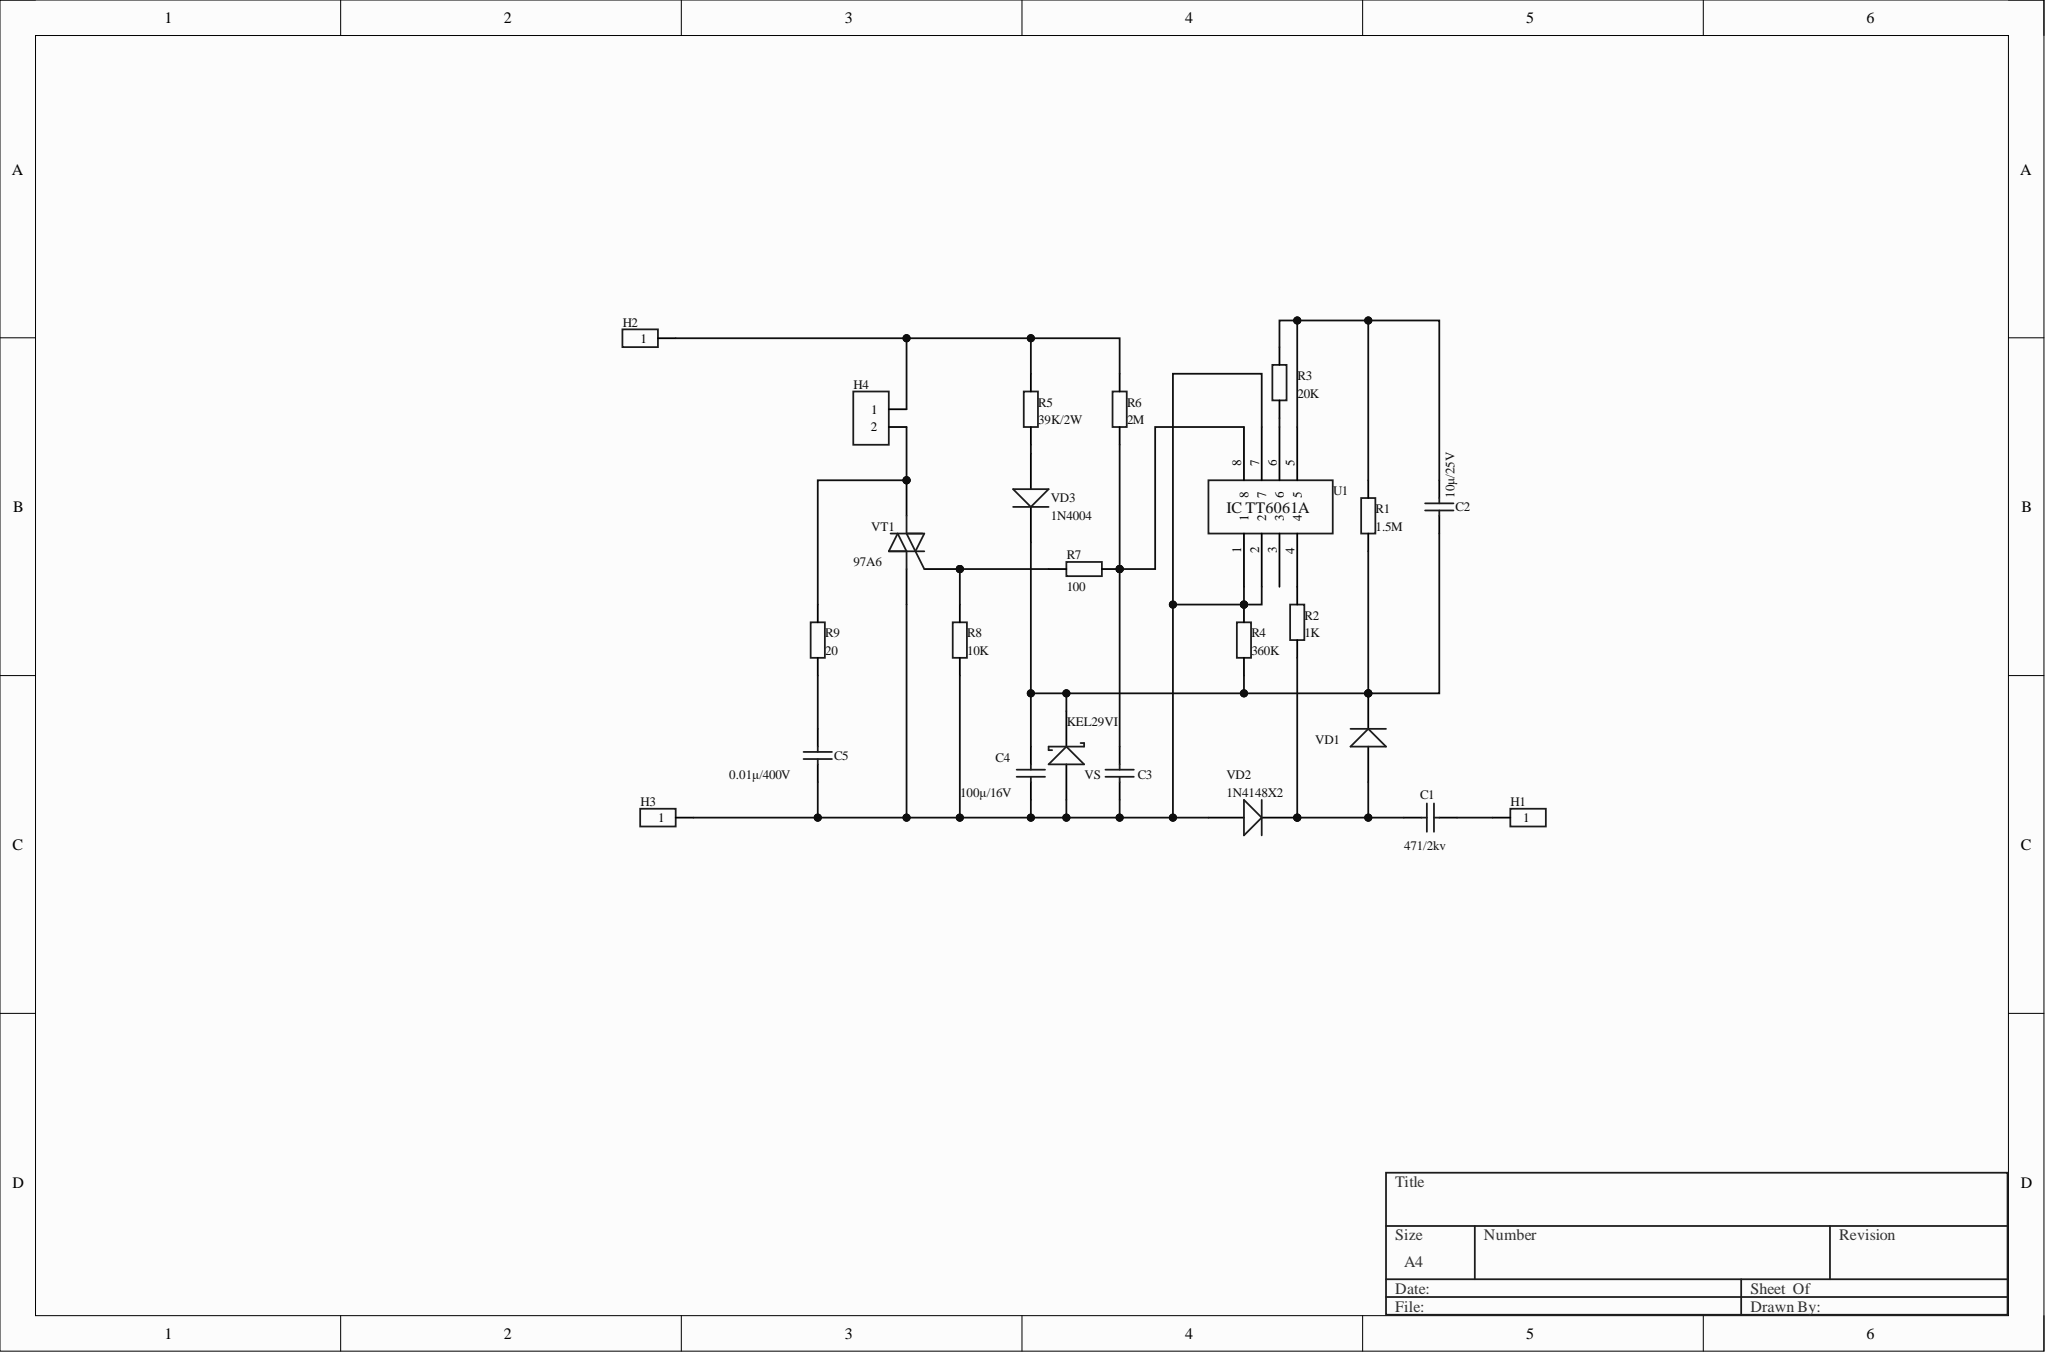Circuit board | Altium Designer | 24 parts | 13 nets
Bill of materials:
Comment,Description,Designator,Footprint,LibRef,Quantity
"","Capacitor","C1, C2, C3, C4, C5","RAD-0.3","Cap","5"
"","","H1, H2, H3","HDR-TH_1P-V-M_XKB_X4611WV-01I-C28D40","HDR-M_2.54_1x1P","3"
"","","H4","HDR-TH_2P-P2.54-V-F","HDR-F_2.54_1x2P","1"
"1.5M","Resistor","R1","Res_1/4W","1.5M","1"
"1K","Resistor","R2","Res_1/4W","1K","1"
"20K","Resistor","R3","Res_1/4W","20K","1"
"360K","Resistor","R4","Res_1/4W","360K","1"
"39K/2W","Resistor","R5","Res_1/4W","10K","1"
"2M","Resistor","R6","Res_1/4W","10K","1"
"100","Resistor","R7","Res_1/4W","360K","1"
"10K","Resistor","R8","Res_1/4W","10K","1"
"20","Resistor","R9","Res_1/4W","20","1"
"","","U1","DIP-8_L9.2-W6.6-P2.54-LS7.62-BL","Component_1","1"
"","Silicon Low Leakage Diode","VD1","DO-41_BD2.4-L4.7-P8.70-D0.9-RD","Diode BAS116","1"
"1N4148X2","Silicon Low Leakage Diode","VD2","DO-41_BD2.4-L4.7-P8.70-D0.9-RD","1N4148X2","1"
"1N4004","Silicon Low Leakage Diode","VD3","DO-41_BD2.4-L4.7-P8.70-D0.9-RD","1N4148X2","1"
"KEL29VI","Schottky Rectifier","VS","DO-41_BD2.4-L4.7-P8.70-D0.9-RD","KEL29VI","1"
"97A6","Silicon Bidirectional Triode Thyristor","VT1","SOT-23-3_L2.9-W1.6-P1.90-LS2.8-BR","97A6","1"
Netlist (Protel format):
[
C1
RAD-0.3




]
[
C2
RAD-0.3




]
[
C3
RAD-0.3




]
[
C4
RAD-0.3




]
[
C5
RAD-0.3




]
[
H1
HDR-TH_1P-V-M_XKB_X4611WV-01I-C28D40




]
[
H2
HDR-TH_1P-V-M_XKB_X4611WV-01I-C28D40




]
[
H3
HDR-TH_1P-V-M_XKB_X4611WV-01I-C28D40




]
[
H4
HDR-TH_2P-P2.54-V-F




]
[
R1
Res_1/4W
1.5M



]
[
R2
Res_1/4W
1K



]
[
R3
Res_1/4W
20K



]
[
R4
Res_1/4W
360K



]
[
R5
Res_1/4W
39K/2W



]
[
R6
Res_1/4W
2M



]
[
R7
Res_1/4W
100



]
[
R8
Res_1/4W
10K



]
[
R9
Res_1/4W
20



]
[
U1
DIP-8_L9.2-W6.6-P2.54-LS7.62-BL




]
[
VD1
DO-41_BD2.4-L4.7-P8.70-D0.9-RD




]
[
VD2
DO-41_BD2.4-L4.7-P8.70-D0.9-RD
1N4148X2



]
[
VD3
DO-41_BD2.4-L4.7-P8.70-D0.9-RD
1N4004



]
[
VS
DO-41_BD2.4-L4.7-P8.70-D0.9-RD
KEL29VI



]
[
VT1
SOT-23-3_L2.9-W1.6-P1.90-LS2.8-BR
97A6



]
(
NetR7_2
R7-2
R8-2
VT1-3
)
(
NetR5_1
R5-1
VD3-1
)
(
NetR3_1
R3-1
U1-6
)
(
NetR2_2
R2-2
U1-4
)
(
NetH4_2
H4-2
R9-2
VT1-2
)
(
NetH2_1
H2-1
H4-1
R5-2
R6-2
)
(
NetC5_2
C5-2
R9-1
)
(
NetC3_2
C3-2
R6-1
R7-1
U1-8
)
(
NetC3_1
C3-1
C4-1
C5-1
H3-1
R4-2
R8-1
U1-1
U1-2
U1-7
VD2-1
VS-3
VT1-1
)
(
NetC2_2
C2-2
R1-2
R3-2
U1-5
)
(
NetC2_1
C2-1
C4-2
R1-1
R4-1
VD1-3
VD3-3
VS-1
)
(
NetC1_2
C1-2
H1-1
)
(
NetC1_1
C1-1
R2-1
VD1-1
VD2-3
)